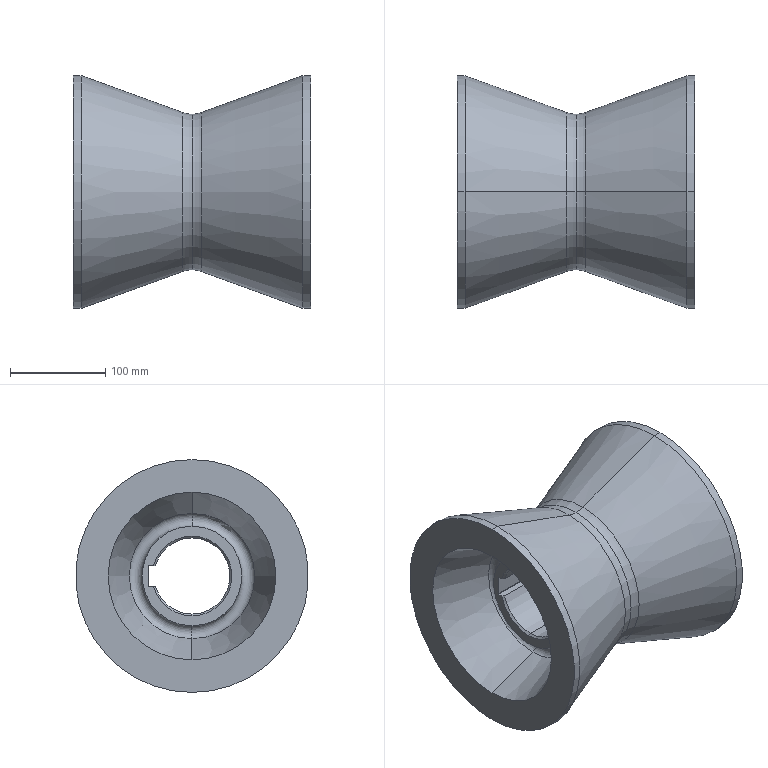Part | SolidWorks | features Chamfer 1, Fillet 1, ICE 1, Revolution 1 | 1 solid | 42 faces | box 250 x 245 x 245 mm | volume 5466955 mm3 | cone 14 | cylinder 13 | torus 8 | plane 7 | commonest cylinder face diameters 105 x4 245 x4 80 x3 1 x2
STEP:
#1=CARTESIAN_POINT('',(-10.261,0.,83.735));
#2=VERTEX_POINT('',#1);
#3=CARTESIAN_POINT('',(0.,0.,81.925));
#4=VERTEX_POINT('',#3);
#5=CARTESIAN_POINT('',(0.,0.,111.925));
#6=DIRECTION('',(0.,-1.,0.));
#7=DIRECTION('',(0.,0.,-1.));
#8=AXIS2_PLACEMENT_3D('',#5,#6,#7);
#9=CIRCLE('',#8,30.);
#10=EDGE_CURVE('',#2,#4,#9,.T.);
#11=ORIENTED_EDGE('',*,*,#10,.T.);
#12=CARTESIAN_POINT('',(0.,0.,-81.925));
#13=VERTEX_POINT('',#12);
#14=CARTESIAN_POINT('',(0.,0.,0.));
#15=DIRECTION('',(-1.,0.,0.));
#16=DIRECTION('',(0.,0.,1.));
#17=AXIS2_PLACEMENT_3D('',#14,#15,#16);
#18=CIRCLE('',#17,81.925);
#19=EDGE_CURVE('',#4,#13,#18,.T.);
#20=ORIENTED_EDGE('',*,*,#19,.T.);
#21=CARTESIAN_POINT('',(-10.261,0.,-83.735));
#22=VERTEX_POINT('',#21);
#23=CARTESIAN_POINT('',(0.,0.,-111.925));
#24=DIRECTION('',(0.,1.,0.));
#25=DIRECTION('',(0.,0.,1.));
#26=AXIS2_PLACEMENT_3D('',#23,#24,#25);
#27=CIRCLE('',#26,30.);
#28=EDGE_CURVE('',#22,#13,#27,.T.);
#29=ORIENTED_EDGE('',*,*,#28,.F.);
#30=CARTESIAN_POINT('',(-10.261,0.,0.));
#31=DIRECTION('',(-1.,0.,0.));
#32=DIRECTION('',(0.,0.,1.));
#33=AXIS2_PLACEMENT_3D('',#30,#31,#32);
#34=CIRCLE('',#33,83.735);
#35=EDGE_CURVE('',#2,#22,#34,.T.);
#36=ORIENTED_EDGE('',*,*,#35,.F.);
#37=EDGE_LOOP('',(#11,#20,#29,#36));
#38=FACE_OUTER_BOUND('',#37,.T.);
#39=CARTESIAN_POINT('',(0.,0.,0.));
#40=DIRECTION('',(-1.,0.,0.));
#41=DIRECTION('',(0.,0.,1.));
#42=AXIS2_PLACEMENT_3D('',#39,#40,#41);
#43=TOROIDAL_SURFACE('',#42,111.925,30.);
#44=ADVANCED_FACE('',(#38),#43,.F.);
#45=ORIENTED_EDGE('',*,*,#28,.T.);
#46=CARTESIAN_POINT('',(0.,0.,0.));
#47=DIRECTION('',(-1.,0.,0.));
#48=DIRECTION('',(0.,0.,1.));
#49=AXIS2_PLACEMENT_3D('',#46,#47,#48);
#50=CIRCLE('',#49,81.925);
#51=EDGE_CURVE('',#13,#4,#50,.T.);
#52=ORIENTED_EDGE('',*,*,#51,.T.);
#53=ORIENTED_EDGE('',*,*,#10,.F.);
#54=CARTESIAN_POINT('',(-10.261,0.,0.));
#55=DIRECTION('',(-1.,0.,0.));
#56=DIRECTION('',(0.,0.,1.));
#57=AXIS2_PLACEMENT_3D('',#54,#55,#56);
#58=CIRCLE('',#57,83.735);
#59=EDGE_CURVE('',#22,#2,#58,.T.);
#60=ORIENTED_EDGE('',*,*,#59,.F.);
#61=EDGE_LOOP('',(#45,#52,#53,#60));
#62=FACE_OUTER_BOUND('',#61,.T.);
#63=CARTESIAN_POINT('',(0.,0.,0.));
#64=DIRECTION('',(-1.,0.,0.));
#65=DIRECTION('',(0.,0.,1.));
#66=AXIS2_PLACEMENT_3D('',#63,#64,#65);
#67=TOROIDAL_SURFACE('',#66,111.925,30.);
#68=ADVANCED_FACE('',(#62),#67,.F.);
#69=CARTESIAN_POINT('',(-68.,0.,-40.));
#70=VERTEX_POINT('',#69);
#71=CARTESIAN_POINT('',(-68.,0.,40.));
#72=VERTEX_POINT('',#71);
#73=CARTESIAN_POINT('',(-68.,0.,0.));
#74=DIRECTION('',(-1.,0.,0.));
#75=DIRECTION('',(0.,0.,-1.));
#76=AXIS2_PLACEMENT_3D('',#73,#74,#75);
#77=CIRCLE('',#76,40.);
#78=EDGE_CURVE('',#70,#72,#77,.T.);
#79=ORIENTED_EDGE('',*,*,#78,.F.);
#80=CARTESIAN_POINT('',(-70.,0.,-42.));
#81=VERTEX_POINT('',#80);
#82=CARTESIAN_POINT('',(-68.,0.,-40.));
#83=DIRECTION('',(-0.7071,0.,-0.7071));
#84=VECTOR('',#83,1000.);
#85=LINE('',#82,#84);
#86=EDGE_CURVE('',#70,#81,#85,.T.);
#87=ORIENTED_EDGE('',*,*,#86,.T.);
#88=CARTESIAN_POINT('',(-70.,0.,42.));
#89=VERTEX_POINT('',#88);
#90=CARTESIAN_POINT('',(-70.,0.,0.));
#91=DIRECTION('',(1.,0.,0.));
#92=DIRECTION('',(0.,0.,-1.));
#93=AXIS2_PLACEMENT_3D('',#90,#91,#92);
#94=CIRCLE('',#93,42.);
#95=EDGE_CURVE('',#89,#81,#94,.T.);
#96=ORIENTED_EDGE('',*,*,#95,.F.);
#97=CARTESIAN_POINT('',(-68.,0.,40.));
#98=DIRECTION('',(-0.7071,0.,0.7071));
#99=VECTOR('',#98,1000.);
#100=LINE('',#97,#99);
#101=EDGE_CURVE('',#72,#89,#100,.T.);
#102=ORIENTED_EDGE('',*,*,#101,.F.);
#103=EDGE_LOOP('',(#79,#87,#96,#102));
#104=FACE_OUTER_BOUND('',#103,.T.);
#105=CARTESIAN_POINT('',(-68.,0.,0.));
#106=DIRECTION('',(-1.,0.,0.));
#107=DIRECTION('',(0.,0.,1.));
#108=AXIS2_PLACEMENT_3D('',#105,#106,#107);
#109=CONICAL_SURFACE('',#108,40.,0.7854);
#110=ADVANCED_FACE('',(#104),#109,.F.);
#111=CARTESIAN_POINT('',(-68.,38.458,11.));
#112=VERTEX_POINT('',#111);
#113=CARTESIAN_POINT('',(-68.,0.,0.));
#114=DIRECTION('',(-1.,0.,0.));
#115=DIRECTION('',(0.,0.,-1.));
#116=AXIS2_PLACEMENT_3D('',#113,#114,#115);
#117=CIRCLE('',#116,40.);
#118=EDGE_CURVE('',#72,#112,#117,.T.);
#119=ORIENTED_EDGE('',*,*,#118,.F.);
#120=ORIENTED_EDGE('',*,*,#101,.T.);
#121=CARTESIAN_POINT('',(-70.,40.534,11.));
#122=VERTEX_POINT('',#121);
#123=CARTESIAN_POINT('',(-70.,0.,0.));
#124=DIRECTION('',(1.,0.,0.));
#125=DIRECTION('',(0.,0.,-1.));
#126=AXIS2_PLACEMENT_3D('',#123,#124,#125);
#127=CIRCLE('',#126,42.);
#128=EDGE_CURVE('',#122,#89,#127,.T.);
#129=ORIENTED_EDGE('',*,*,#128,.F.);
#130=CARTESIAN_POINT('',(-68.,38.458,11.));
#131=CARTESIAN_POINT('',(-68.666,39.15,11.));
#132=CARTESIAN_POINT('',(-69.333,39.842,11.));
#133=CARTESIAN_POINT('',(-70.,40.534,11.));
#134=B_SPLINE_CURVE_WITH_KNOTS('',3,(#130,#131,#132,#133),.UNSPECIFIED.,.F.,.F.,(4,4),(0.,0.002883),.UNSPECIFIED.);
#135=EDGE_CURVE('',#112,#122,#134,.T.);
#136=ORIENTED_EDGE('',*,*,#135,.F.);
#137=EDGE_LOOP('',(#119,#120,#129,#136));
#138=FACE_OUTER_BOUND('',#137,.T.);
#139=CARTESIAN_POINT('',(-68.,0.,0.));
#140=DIRECTION('',(-1.,0.,0.));
#141=DIRECTION('',(0.,0.,1.));
#142=AXIS2_PLACEMENT_3D('',#139,#140,#141);
#143=CONICAL_SURFACE('',#142,40.,0.7854);
#144=ADVANCED_FACE('',(#138),#143,.F.);
#145=CARTESIAN_POINT('',(68.,0.,40.));
#146=VERTEX_POINT('',#145);
#147=CARTESIAN_POINT('',(68.,0.,-40.));
#148=VERTEX_POINT('',#147);
#149=CARTESIAN_POINT('',(68.,0.,0.));
#150=DIRECTION('',(1.,0.,0.));
#151=DIRECTION('',(0.,0.,1.));
#152=AXIS2_PLACEMENT_3D('',#149,#150,#151);
#153=CIRCLE('',#152,40.);
#154=EDGE_CURVE('',#146,#148,#153,.T.);
#155=ORIENTED_EDGE('',*,*,#154,.F.);
#156=CARTESIAN_POINT('',(70.,0.,42.));
#157=VERTEX_POINT('',#156);
#158=CARTESIAN_POINT('',(70.,0.,42.));
#159=DIRECTION('',(0.7071,0.,0.7071));
#160=VECTOR('',#159,1000.);
#161=LINE('',#158,#160);
#162=EDGE_CURVE('',#146,#157,#161,.T.);
#163=ORIENTED_EDGE('',*,*,#162,.T.);
#164=CARTESIAN_POINT('',(70.,0.,-42.));
#165=VERTEX_POINT('',#164);
#166=CARTESIAN_POINT('',(70.,0.,0.));
#167=DIRECTION('',(-1.,0.,0.));
#168=DIRECTION('',(0.,0.,1.));
#169=AXIS2_PLACEMENT_3D('',#166,#167,#168);
#170=CIRCLE('',#169,42.);
#171=EDGE_CURVE('',#165,#157,#170,.T.);
#172=ORIENTED_EDGE('',*,*,#171,.F.);
#173=CARTESIAN_POINT('',(70.,0.,-42.));
#174=DIRECTION('',(0.7071,0.,-0.7071));
#175=VECTOR('',#174,1000.);
#176=LINE('',#173,#175);
#177=EDGE_CURVE('',#148,#165,#176,.T.);
#178=ORIENTED_EDGE('',*,*,#177,.F.);
#179=EDGE_LOOP('',(#155,#163,#172,#178));
#180=FACE_OUTER_BOUND('',#179,.T.);
#181=CARTESIAN_POINT('',(70.,0.,0.));
#182=DIRECTION('',(1.,0.,0.));
#183=DIRECTION('',(0.,0.,-1.));
#184=AXIS2_PLACEMENT_3D('',#181,#182,#183);
#185=CONICAL_SURFACE('',#184,42.,0.7854);
#186=ADVANCED_FACE('',(#180),#185,.F.);
#187=CARTESIAN_POINT('',(68.,38.458,-11.));
#188=VERTEX_POINT('',#187);
#189=CARTESIAN_POINT('',(68.,0.,0.));
#190=DIRECTION('',(1.,0.,0.));
#191=DIRECTION('',(0.,0.,1.));
#192=AXIS2_PLACEMENT_3D('',#189,#190,#191);
#193=CIRCLE('',#192,40.);
#194=EDGE_CURVE('',#148,#188,#193,.T.);
#195=ORIENTED_EDGE('',*,*,#194,.F.);
#196=ORIENTED_EDGE('',*,*,#177,.T.);
#197=CARTESIAN_POINT('',(70.,40.534,-11.));
#198=VERTEX_POINT('',#197);
#199=CARTESIAN_POINT('',(70.,0.,0.));
#200=DIRECTION('',(-1.,0.,0.));
#201=DIRECTION('',(0.,0.,1.));
#202=AXIS2_PLACEMENT_3D('',#199,#200,#201);
#203=CIRCLE('',#202,42.);
#204=EDGE_CURVE('',#198,#165,#203,.T.);
#205=ORIENTED_EDGE('',*,*,#204,.F.);
#206=CARTESIAN_POINT('',(68.,38.458,-11.));
#207=CARTESIAN_POINT('',(68.666,39.15,-11.));
#208=CARTESIAN_POINT('',(69.333,39.842,-11.));
#209=CARTESIAN_POINT('',(70.,40.534,-11.));
#210=B_SPLINE_CURVE_WITH_KNOTS('',3,(#206,#207,#208,#209),.UNSPECIFIED.,.F.,.F.,(4,4),(0.,0.002883),.UNSPECIFIED.);
#211=EDGE_CURVE('',#188,#198,#210,.T.);
#212=ORIENTED_EDGE('',*,*,#211,.F.);
#213=EDGE_LOOP('',(#195,#196,#205,#212));
#214=FACE_OUTER_BOUND('',#213,.T.);
#215=CARTESIAN_POINT('',(70.,0.,0.));
#216=DIRECTION('',(1.,0.,0.));
#217=DIRECTION('',(0.,0.,-1.));
#218=AXIS2_PLACEMENT_3D('',#215,#216,#217);
#219=CONICAL_SURFACE('',#218,42.,0.7854);
#220=ADVANCED_FACE('',(#214),#219,.F.);
#221=ORIENTED_EDGE('',*,*,#154,.T.);
#222=CARTESIAN_POINT('',(125.,0.,-40.));
#223=DIRECTION('',(-1.,0.,0.));
#224=VECTOR('',#223,1000.);
#225=LINE('',#222,#224);
#226=EDGE_CURVE('',#148,#70,#225,.T.);
#227=ORIENTED_EDGE('',*,*,#226,.T.);
#228=ORIENTED_EDGE('',*,*,#78,.T.);
#229=CARTESIAN_POINT('',(125.,0.,40.));
#230=DIRECTION('',(-1.,0.,0.));
#231=VECTOR('',#230,1000.);
#232=LINE('',#229,#231);
#233=EDGE_CURVE('',#146,#72,#232,.T.);
#234=ORIENTED_EDGE('',*,*,#233,.F.);
#235=EDGE_LOOP('',(#221,#227,#228,#234));
#236=FACE_OUTER_BOUND('',#235,.T.);
#237=CARTESIAN_POINT('',(125.,0.,0.));
#238=DIRECTION('',(-1.,0.,0.));
#239=DIRECTION('',(0.,0.,1.));
#240=AXIS2_PLACEMENT_3D('',#237,#238,#239);
#241=CYLINDRICAL_SURFACE('',#240,40.);
#242=ADVANCED_FACE('',(#236),#241,.F.);
#243=CARTESIAN_POINT('',(68.,38.458,11.));
#244=VERTEX_POINT('',#243);
#245=CARTESIAN_POINT('',(68.,0.,0.));
#246=DIRECTION('',(1.,0.,0.));
#247=DIRECTION('',(0.,0.,1.));
#248=AXIS2_PLACEMENT_3D('',#245,#246,#247);
#249=CIRCLE('',#248,40.);
#250=EDGE_CURVE('',#244,#146,#249,.T.);
#251=ORIENTED_EDGE('',*,*,#250,.T.);
#252=ORIENTED_EDGE('',*,*,#233,.T.);
#253=ORIENTED_EDGE('',*,*,#118,.T.);
#254=CARTESIAN_POINT('',(125.,38.458,11.));
#255=DIRECTION('',(-1.,0.,0.));
#256=VECTOR('',#255,1000.);
#257=LINE('',#254,#256);
#258=EDGE_CURVE('',#244,#112,#257,.T.);
#259=ORIENTED_EDGE('',*,*,#258,.F.);
#260=EDGE_LOOP('',(#251,#252,#253,#259));
#261=FACE_OUTER_BOUND('',#260,.T.);
#262=CARTESIAN_POINT('',(125.,0.,0.));
#263=DIRECTION('',(-1.,0.,0.));
#264=DIRECTION('',(0.,0.,1.));
#265=AXIS2_PLACEMENT_3D('',#262,#263,#264);
#266=CYLINDRICAL_SURFACE('',#265,40.);
#267=ADVANCED_FACE('',(#261),#266,.F.);
#268=CARTESIAN_POINT('',(-66.476,0.,-52.5));
#269=VERTEX_POINT('',#268);
#270=CARTESIAN_POINT('',(-66.476,0.,52.5));
#271=VERTEX_POINT('',#270);
#272=CARTESIAN_POINT('',(-66.476,0.,0.));
#273=DIRECTION('',(-1.,0.,0.));
#274=DIRECTION('',(0.,0.,1.));
#275=AXIS2_PLACEMENT_3D('',#272,#273,#274);
#276=CIRCLE('',#275,52.5);
#277=EDGE_CURVE('',#269,#271,#276,.T.);
#278=ORIENTED_EDGE('',*,*,#277,.F.);
#279=CARTESIAN_POINT('',(-64.082,0.,-66.078));
#280=VERTEX_POINT('',#279);
#281=CARTESIAN_POINT('',(-66.476,0.,-59.5));
#282=DIRECTION('',(0.,1.,0.));
#283=DIRECTION('',(0.,0.,1.));
#284=AXIS2_PLACEMENT_3D('',#281,#282,#283);
#285=CIRCLE('',#284,7.);
#286=EDGE_CURVE('',#269,#280,#285,.T.);
#287=ORIENTED_EDGE('',*,*,#286,.T.);
#288=CARTESIAN_POINT('',(-64.082,0.,66.078));
#289=VERTEX_POINT('',#288);
#290=CARTESIAN_POINT('',(-64.082,0.,0.));
#291=DIRECTION('',(-1.,0.,0.));
#292=DIRECTION('',(0.,0.,1.));
#293=AXIS2_PLACEMENT_3D('',#290,#291,#292);
#294=CIRCLE('',#293,66.078);
#295=EDGE_CURVE('',#280,#289,#294,.T.);
#296=ORIENTED_EDGE('',*,*,#295,.T.);
#297=CARTESIAN_POINT('',(-66.476,0.,59.5));
#298=DIRECTION('',(0.,-1.,0.));
#299=DIRECTION('',(0.,0.,-1.));
#300=AXIS2_PLACEMENT_3D('',#297,#298,#299);
#301=CIRCLE('',#300,7.);
#302=EDGE_CURVE('',#271,#289,#301,.T.);
#303=ORIENTED_EDGE('',*,*,#302,.F.);
#304=EDGE_LOOP('',(#278,#287,#296,#303));
#305=FACE_OUTER_BOUND('',#304,.T.);
#306=CARTESIAN_POINT('',(-66.476,0.,0.));
#307=DIRECTION('',(-1.,0.,0.));
#308=DIRECTION('',(0.,0.,1.));
#309=AXIS2_PLACEMENT_3D('',#306,#307,#308);
#310=TOROIDAL_SURFACE('',#309,59.5,7.);
#311=ADVANCED_FACE('',(#305),#310,.F.);
#312=ORIENTED_EDGE('',*,*,#295,.F.);
#313=CARTESIAN_POINT('',(-125.,0.,-88.25));
#314=VERTEX_POINT('',#313);
#315=CARTESIAN_POINT('',(-125.,0.,-88.25));
#316=DIRECTION('',(-0.9397,0.,-0.342));
#317=VECTOR('',#316,1000.);
#318=LINE('',#315,#317);
#319=EDGE_CURVE('',#280,#314,#318,.T.);
#320=ORIENTED_EDGE('',*,*,#319,.T.);
#321=CARTESIAN_POINT('',(-125.,0.,88.25));
#322=VERTEX_POINT('',#321);
#323=CARTESIAN_POINT('',(-125.,0.,0.));
#324=DIRECTION('',(-1.,0.,0.));
#325=DIRECTION('',(0.,0.,1.));
#326=AXIS2_PLACEMENT_3D('',#323,#324,#325);
#327=CIRCLE('',#326,88.25);
#328=EDGE_CURVE('',#314,#322,#327,.T.);
#329=ORIENTED_EDGE('',*,*,#328,.T.);
#330=CARTESIAN_POINT('',(-125.,0.,88.25));
#331=DIRECTION('',(-0.9397,0.,0.342));
#332=VECTOR('',#331,1000.);
#333=LINE('',#330,#332);
#334=EDGE_CURVE('',#289,#322,#333,.T.);
#335=ORIENTED_EDGE('',*,*,#334,.F.);
#336=EDGE_LOOP('',(#312,#320,#329,#335));
#337=FACE_OUTER_BOUND('',#336,.T.);
#338=CARTESIAN_POINT('',(-125.,0.,0.));
#339=DIRECTION('',(-1.,0.,0.));
#340=DIRECTION('',(0.,0.,1.));
#341=AXIS2_PLACEMENT_3D('',#338,#339,#340);
#342=CONICAL_SURFACE('',#341,88.25,0.3491);
#343=ADVANCED_FACE('',(#337),#342,.F.);
#344=CARTESIAN_POINT('',(-116.768,0.,122.5));
#345=VERTEX_POINT('',#344);
#346=CARTESIAN_POINT('',(-116.768,0.,-122.5));
#347=VERTEX_POINT('',#346);
#348=CARTESIAN_POINT('',(-116.768,0.,0.));
#349=DIRECTION('',(-1.,0.,0.));
#350=DIRECTION('',(0.,0.,1.));
#351=AXIS2_PLACEMENT_3D('',#348,#349,#350);
#352=CIRCLE('',#351,122.5);
#353=EDGE_CURVE('',#345,#347,#352,.T.);
#354=ORIENTED_EDGE('',*,*,#353,.T.);
#355=CARTESIAN_POINT('',(-125.,0.,-122.5));
#356=VERTEX_POINT('',#355);
#357=CARTESIAN_POINT('',(-70.,0.,-122.5));
#358=DIRECTION('',(-1.,0.,0.));
#359=VECTOR('',#358,1000.);
#360=LINE('',#357,#359);
#361=EDGE_CURVE('',#347,#356,#360,.T.);
#362=ORIENTED_EDGE('',*,*,#361,.T.);
#363=CARTESIAN_POINT('',(-125.,0.,122.5));
#364=VERTEX_POINT('',#363);
#365=CARTESIAN_POINT('',(-125.,0.,0.));
#366=DIRECTION('',(-1.,0.,0.));
#367=DIRECTION('',(0.,0.,1.));
#368=AXIS2_PLACEMENT_3D('',#365,#366,#367);
#369=CIRCLE('',#368,122.5);
#370=EDGE_CURVE('',#364,#356,#369,.T.);
#371=ORIENTED_EDGE('',*,*,#370,.F.);
#372=CARTESIAN_POINT('',(-70.,0.,122.5));
#373=DIRECTION('',(-1.,0.,0.));
#374=VECTOR('',#373,1000.);
#375=LINE('',#372,#374);
#376=EDGE_CURVE('',#345,#364,#375,.T.);
#377=ORIENTED_EDGE('',*,*,#376,.F.);
#378=EDGE_LOOP('',(#354,#362,#371,#377));
#379=FACE_OUTER_BOUND('',#378,.T.);
#380=CARTESIAN_POINT('',(-70.,0.,0.));
#381=DIRECTION('',(-1.,0.,0.));
#382=DIRECTION('',(0.,0.,1.));
#383=AXIS2_PLACEMENT_3D('',#380,#381,#382);
#384=CYLINDRICAL_SURFACE('',#383,122.5);
#385=ADVANCED_FACE('',(#379),#384,.T.);
#386=ORIENTED_EDGE('',*,*,#35,.T.);
#387=CARTESIAN_POINT('',(-10.261,0.,-83.735));
#388=DIRECTION('',(-0.9397,0.,-0.342));
#389=VECTOR('',#388,1000.);
#390=LINE('',#387,#389);
#391=EDGE_CURVE('',#22,#347,#390,.T.);
#392=ORIENTED_EDGE('',*,*,#391,.T.);
#393=ORIENTED_EDGE('',*,*,#353,.F.);
#394=CARTESIAN_POINT('',(-10.261,0.,83.735));
#395=DIRECTION('',(-0.9397,0.,0.342));
#396=VECTOR('',#395,1000.);
#397=LINE('',#394,#396);
#398=EDGE_CURVE('',#2,#345,#397,.T.);
#399=ORIENTED_EDGE('',*,*,#398,.F.);
#400=EDGE_LOOP('',(#386,#392,#393,#399));
#401=FACE_OUTER_BOUND('',#400,.T.);
#402=CARTESIAN_POINT('',(-10.261,0.,0.));
#403=DIRECTION('',(-1.,0.,0.));
#404=DIRECTION('',(0.,0.,1.));
#405=AXIS2_PLACEMENT_3D('',#402,#403,#404);
#406=CONICAL_SURFACE('',#405,83.735,0.3491);
#407=ADVANCED_FACE('',(#401),#406,.T.);
#408=ORIENTED_EDGE('',*,*,#51,.F.);
#409=CARTESIAN_POINT('',(10.261,0.,-83.735));
#410=VERTEX_POINT('',#409);
#411=CARTESIAN_POINT('',(0.,0.,-111.925));
#412=DIRECTION('',(0.,1.,0.));
#413=DIRECTION('',(0.,0.,1.));
#414=AXIS2_PLACEMENT_3D('',#411,#412,#413);
#415=CIRCLE('',#414,30.);
#416=EDGE_CURVE('',#13,#410,#415,.T.);
#417=ORIENTED_EDGE('',*,*,#416,.T.);
#418=CARTESIAN_POINT('',(10.261,0.,83.735));
#419=VERTEX_POINT('',#418);
#420=CARTESIAN_POINT('',(10.261,0.,0.));
#421=DIRECTION('',(-1.,0.,0.));
#422=DIRECTION('',(0.,0.,1.));
#423=AXIS2_PLACEMENT_3D('',#420,#421,#422);
#424=CIRCLE('',#423,83.735);
#425=EDGE_CURVE('',#410,#419,#424,.T.);
#426=ORIENTED_EDGE('',*,*,#425,.T.);
#427=CARTESIAN_POINT('',(0.,0.,111.925));
#428=DIRECTION('',(0.,-1.,0.));
#429=DIRECTION('',(0.,0.,-1.));
#430=AXIS2_PLACEMENT_3D('',#427,#428,#429);
#431=CIRCLE('',#430,30.);
#432=EDGE_CURVE('',#4,#419,#431,.T.);
#433=ORIENTED_EDGE('',*,*,#432,.F.);
#434=EDGE_LOOP('',(#408,#417,#426,#433));
#435=FACE_OUTER_BOUND('',#434,.T.);
#436=CARTESIAN_POINT('',(0.,0.,0.));
#437=DIRECTION('',(-1.,0.,0.));
#438=DIRECTION('',(0.,0.,1.));
#439=AXIS2_PLACEMENT_3D('',#436,#437,#438);
#440=TOROIDAL_SURFACE('',#439,111.925,30.);
#441=ADVANCED_FACE('',(#435),#440,.F.);
#442=CARTESIAN_POINT('',(10.261,0.,0.));
#443=DIRECTION('',(-1.,0.,0.));
#444=DIRECTION('',(0.,0.,1.));
#445=AXIS2_PLACEMENT_3D('',#442,#443,#444);
#446=CIRCLE('',#445,83.735);
#447=EDGE_CURVE('',#419,#410,#446,.T.);
#448=ORIENTED_EDGE('',*,*,#447,.F.);
#449=CARTESIAN_POINT('',(116.768,0.,122.5));
#450=VERTEX_POINT('',#449);
#451=CARTESIAN_POINT('',(116.768,0.,122.5));
#452=DIRECTION('',(0.9397,0.,0.342));
#453=VECTOR('',#452,1000.);
#454=LINE('',#451,#453);
#455=EDGE_CURVE('',#419,#450,#454,.T.);
#456=ORIENTED_EDGE('',*,*,#455,.T.);
#457=CARTESIAN_POINT('',(116.768,0.,-122.5));
#458=VERTEX_POINT('',#457);
#459=CARTESIAN_POINT('',(116.768,0.,0.));
#460=DIRECTION('',(-1.,0.,0.));
#461=DIRECTION('',(0.,0.,1.));
#462=AXIS2_PLACEMENT_3D('',#459,#460,#461);
#463=CIRCLE('',#462,122.5);
#464=EDGE_CURVE('',#450,#458,#463,.T.);
#465=ORIENTED_EDGE('',*,*,#464,.T.);
#466=CARTESIAN_POINT('',(116.768,0.,-122.5));
#467=DIRECTION('',(0.9397,0.,-0.342));
#468=VECTOR('',#467,1000.);
#469=LINE('',#466,#468);
#470=EDGE_CURVE('',#410,#458,#469,.T.);
#471=ORIENTED_EDGE('',*,*,#470,.F.);
#472=EDGE_LOOP('',(#448,#456,#465,#471));
#473=FACE_OUTER_BOUND('',#472,.T.);
#474=CARTESIAN_POINT('',(116.768,0.,0.));
#475=DIRECTION('',(1.,0.,0.));
#476=DIRECTION('',(0.,0.,-1.));
#477=AXIS2_PLACEMENT_3D('',#474,#475,#476);
#478=CONICAL_SURFACE('',#477,122.5,0.3491);
#479=ADVANCED_FACE('',(#473),#478,.T.);
#480=CARTESIAN_POINT('',(125.,0.,122.5));
#481=VERTEX_POINT('',#480);
#482=CARTESIAN_POINT('',(125.,0.,-122.5));
#483=VERTEX_POINT('',#482);
#484=CARTESIAN_POINT('',(125.,0.,0.));
#485=DIRECTION('',(-1.,0.,0.));
#486=DIRECTION('',(0.,0.,1.));
#487=AXIS2_PLACEMENT_3D('',#484,#485,#486);
#488=CIRCLE('',#487,122.5);
#489=EDGE_CURVE('',#481,#483,#488,.T.);
#490=ORIENTED_EDGE('',*,*,#489,.T.);
#491=CARTESIAN_POINT('',(-70.,0.,-122.5));
#492=DIRECTION('',(-1.,0.,0.));
#493=VECTOR('',#492,1000.);
#494=LINE('',#491,#493);
#495=EDGE_CURVE('',#483,#458,#494,.T.);
#496=ORIENTED_EDGE('',*,*,#495,.T.);
#497=ORIENTED_EDGE('',*,*,#464,.F.);
#498=CARTESIAN_POINT('',(-70.,0.,122.5));
#499=DIRECTION('',(-1.,0.,0.));
#500=VECTOR('',#499,1000.);
#501=LINE('',#498,#500);
#502=EDGE_CURVE('',#481,#450,#501,.T.);
#503=ORIENTED_EDGE('',*,*,#502,.F.);
#504=EDGE_LOOP('',(#490,#496,#497,#503));
#505=FACE_OUTER_BOUND('',#504,.T.);
#506=CARTESIAN_POINT('',(-70.,0.,0.));
#507=DIRECTION('',(-1.,0.,0.));
#508=DIRECTION('',(0.,0.,1.));
#509=AXIS2_PLACEMENT_3D('',#506,#507,#508);
#510=CYLINDRICAL_SURFACE('',#509,122.5);
#511=ADVANCED_FACE('',(#505),#510,.T.);
#512=CARTESIAN_POINT('',(64.082,0.,-66.078));
#513=VERTEX_POINT('',#512);
#514=CARTESIAN_POINT('',(64.082,0.,66.078));
#515=VERTEX_POINT('',#514);
#516=CARTESIAN_POINT('',(64.082,0.,0.));
#517=DIRECTION('',(-1.,0.,0.));
#518=DIRECTION('',(0.,0.,1.));
#519=AXIS2_PLACEMENT_3D('',#516,#517,#518);
#520=CIRCLE('',#519,66.078);
#521=EDGE_CURVE('',#513,#515,#520,.T.);
#522=ORIENTED_EDGE('',*,*,#521,.T.);
#523=CARTESIAN_POINT('',(125.,0.,88.25));
#524=VERTEX_POINT('',#523);
#525=CARTESIAN_POINT('',(64.082,0.,66.078));
#526=DIRECTION('',(0.9397,0.,0.342));
#527=VECTOR('',#526,1000.);
#528=LINE('',#525,#527);
#529=EDGE_CURVE('',#515,#524,#528,.T.);
#530=ORIENTED_EDGE('',*,*,#529,.T.);
#531=CARTESIAN_POINT('',(125.,0.,-88.25));
#532=VERTEX_POINT('',#531);
#533=CARTESIAN_POINT('',(125.,0.,0.));
#534=DIRECTION('',(-1.,0.,0.));
#535=DIRECTION('',(0.,0.,1.));
#536=AXIS2_PLACEMENT_3D('',#533,#534,#535);
#537=CIRCLE('',#536,88.25);
#538=EDGE_CURVE('',#532,#524,#537,.T.);
#539=ORIENTED_EDGE('',*,*,#538,.F.);
#540=CARTESIAN_POINT('',(64.082,0.,-66.078));
#541=DIRECTION('',(0.9397,0.,-0.342));
#542=VECTOR('',#541,1000.);
#543=LINE('',#540,#542);
#544=EDGE_CURVE('',#513,#532,#543,.T.);
#545=ORIENTED_EDGE('',*,*,#544,.F.);
#546=EDGE_LOOP('',(#522,#530,#539,#545));
#547=FACE_OUTER_BOUND('',#546,.T.);
#548=CARTESIAN_POINT('',(64.082,0.,0.));
#549=DIRECTION('',(1.,0.,0.));
#550=DIRECTION('',(0.,0.,-1.));
#551=AXIS2_PLACEMENT_3D('',#548,#549,#550);
#552=CONICAL_SURFACE('',#551,66.078,0.3491);
#553=ADVANCED_FACE('',(#547),#552,.F.);
#554=ORIENTED_EDGE('',*,*,#521,.F.);
#555=CARTESIAN_POINT('',(66.476,0.,-52.5));
#556=VERTEX_POINT('',#555);
#557=CARTESIAN_POINT('',(66.476,0.,-59.5));
#558=DIRECTION('',(0.,1.,0.));
#559=DIRECTION('',(0.,0.,1.));
#560=AXIS2_PLACEMENT_3D('',#557,#558,#559);
#561=CIRCLE('',#560,7.);
#562=EDGE_CURVE('',#513,#556,#561,.T.);
#563=ORIENTED_EDGE('',*,*,#562,.T.);
#564=CARTESIAN_POINT('',(66.476,0.,52.5));
#565=VERTEX_POINT('',#564);
#566=CARTESIAN_POINT('',(66.476,0.,0.));
#567=DIRECTION('',(-1.,0.,0.));
#568=DIRECTION('',(0.,0.,1.));
#569=AXIS2_PLACEMENT_3D('',#566,#567,#568);
#570=CIRCLE('',#569,52.5);
#571=EDGE_CURVE('',#556,#565,#570,.T.);
#572=ORIENTED_EDGE('',*,*,#571,.T.);
#573=CARTESIAN_POINT('',(66.476,0.,59.5));
#574=DIRECTION('',(0.,-1.,0.));
#575=DIRECTION('',(0.,0.,-1.));
#576=AXIS2_PLACEMENT_3D('',#573,#574,#575);
#577=CIRCLE('',#576,7.);
#578=EDGE_CURVE('',#515,#565,#577,.T.);
#579=ORIENTED_EDGE('',*,*,#578,.F.);
#580=EDGE_LOOP('',(#554,#563,#572,#579));
#581=FACE_OUTER_BOUND('',#580,.T.);
#582=CARTESIAN_POINT('',(66.476,0.,0.));
#583=DIRECTION('',(-1.,0.,0.));
#584=DIRECTION('',(0.,0.,1.));
#585=AXIS2_PLACEMENT_3D('',#582,#583,#584);
#586=TOROIDAL_SURFACE('',#585,59.5,7.);
#587=ADVANCED_FACE('',(#581),#586,.F.);
#588=CARTESIAN_POINT('',(70.,0.,52.5));
#589=VERTEX_POINT('',#588);
#590=CARTESIAN_POINT('',(70.,0.,-52.5));
#591=VERTEX_POINT('',#590);
#592=CARTESIAN_POINT('',(70.,0.,0.));
#593=DIRECTION('',(-1.,0.,0.));
#594=DIRECTION('',(0.,0.,1.));
#595=AXIS2_PLACEMENT_3D('',#592,#593,#594);
#596=CIRCLE('',#595,52.5);
#597=EDGE_CURVE('',#589,#591,#596,.T.);
#598=ORIENTED_EDGE('',*,*,#597,.T.);
#599=CARTESIAN_POINT('',(-70.,0.,-52.5));
#600=DIRECTION('',(-1.,0.,0.));
#601=VECTOR('',#600,1000.);
#602=LINE('',#599,#601);
#603=EDGE_CURVE('',#591,#556,#602,.T.);
#604=ORIENTED_EDGE('',*,*,#603,.T.);
#605=CARTESIAN_POINT('',(66.476,0.,0.));
#606=DIRECTION('',(-1.,0.,0.));
#607=DIRECTION('',(0.,0.,1.));
#608=AXIS2_PLACEMENT_3D('',#605,#606,#607);
#609=CIRCLE('',#608,52.5);
#610=EDGE_CURVE('',#565,#556,#609,.T.);
#611=ORIENTED_EDGE('',*,*,#610,.F.);
#612=CARTESIAN_POINT('',(-70.,0.,52.5));
#613=DIRECTION('',(-1.,0.,0.));
#614=VECTOR('',#613,1000.);
#615=LINE('',#612,#614);
#616=EDGE_CURVE('',#589,#565,#615,.T.);
#617=ORIENTED_EDGE('',*,*,#616,.F.);
#618=EDGE_LOOP('',(#598,#604,#611,#617));
#619=FACE_OUTER_BOUND('',#618,.T.);
#620=CARTESIAN_POINT('',(-70.,0.,0.));
#621=DIRECTION('',(-1.,0.,0.));
#622=DIRECTION('',(0.,0.,1.));
#623=AXIS2_PLACEMENT_3D('',#620,#621,#622);
#624=CYLINDRICAL_SURFACE('',#623,52.5);
#625=ADVANCED_FACE('',(#619),#624,.T.);
#626=CARTESIAN_POINT('',(-66.476,0.,0.));
#627=DIRECTION('',(-1.,0.,0.));
#628=DIRECTION('',(0.,0.,1.));
#629=AXIS2_PLACEMENT_3D('',#626,#627,#628);
#630=CIRCLE('',#629,52.5);
#631=EDGE_CURVE('',#271,#269,#630,.T.);
#632=ORIENTED_EDGE('',*,*,#631,.T.);
#633=CARTESIAN_POINT('',(-70.,0.,-52.5));
#634=VERTEX_POINT('',#633);
#635=CARTESIAN_POINT('',(-70.,0.,-52.5));
#636=DIRECTION('',(-1.,0.,0.));
#637=VECTOR('',#636,1000.);
#638=LINE('',#635,#637);
#639=EDGE_CURVE('',#269,#634,#638,.T.);
#640=ORIENTED_EDGE('',*,*,#639,.T.);
#641=CARTESIAN_POINT('',(-70.,0.,52.5));
#642=VERTEX_POINT('',#641);
#643=CARTESIAN_POINT('',(-70.,0.,0.));
#644=DIRECTION('',(-1.,0.,0.));
#645=DIRECTION('',(0.,0.,1.));
#646=AXIS2_PLACEMENT_3D('',#643,#644,#645);
#647=CIRCLE('',#646,52.5);
#648=EDGE_CURVE('',#642,#634,#647,.T.);
#649=ORIENTED_EDGE('',*,*,#648,.F.);
#650=CARTESIAN_POINT('',(-70.,0.,52.5));
#651=DIRECTION('',(-1.,0.,0.));
#652=VECTOR('',#651,1000.);
#653=LINE('',#650,#652);
#654=EDGE_CURVE('',#271,#642,#653,.T.);
#655=ORIENTED_EDGE('',*,*,#654,.F.);
#656=EDGE_LOOP('',(#632,#640,#649,#655));
#657=FACE_OUTER_BOUND('',#656,.T.);
#658=CARTESIAN_POINT('',(-70.,0.,0.));
#659=DIRECTION('',(-1.,0.,0.));
#660=DIRECTION('',(0.,0.,1.));
#661=AXIS2_PLACEMENT_3D('',#658,#659,#660);
#662=CYLINDRICAL_SURFACE('',#661,52.5);
#663=ADVANCED_FACE('',(#657),#662,.T.);
#664=ORIENTED_EDGE('',*,*,#639,.F.);
#665=ORIENTED_EDGE('',*,*,#277,.T.);
#666=ORIENTED_EDGE('',*,*,#654,.T.);
#667=CARTESIAN_POINT('',(-70.,0.,0.));
#668=DIRECTION('',(-1.,0.,0.));
#669=DIRECTION('',(0.,0.,1.));
#670=AXIS2_PLACEMENT_3D('',#667,#668,#669);
#671=CIRCLE('',#670,52.5);
#672=EDGE_CURVE('',#634,#642,#671,.T.);
#673=ORIENTED_EDGE('',*,*,#672,.F.);
#674=EDGE_LOOP('',(#664,#665,#666,#673));
#675=FACE_OUTER_BOUND('',#674,.T.);
#676=CARTESIAN_POINT('',(-70.,0.,0.));
#677=DIRECTION('',(-1.,0.,0.));
#678=DIRECTION('',(0.,0.,1.));
#679=AXIS2_PLACEMENT_3D('',#676,#677,#678);
#680=CYLINDRICAL_SURFACE('',#679,52.5);
#681=ADVANCED_FACE('',(#675),#680,.T.);
#682=CARTESIAN_POINT('',(-70.,44.9,11.));
#683=VERTEX_POINT('',#682);
#684=CARTESIAN_POINT('',(-70.,45.4,11.));
#685=DIRECTION('',(0.,1.,0.));
#686=VECTOR('',#685,1000.);
#687=LINE('',#684,#686);
#688=EDGE_CURVE('',#122,#683,#687,.T.);
#689=ORIENTED_EDGE('',*,*,#688,.F.);
#690=ORIENTED_EDGE('',*,*,#128,.T.);
#691=ORIENTED_EDGE('',*,*,#95,.T.);
#692=CARTESIAN_POINT('',(-70.,40.534,-11.));
#693=VERTEX_POINT('',#692);
#694=CARTESIAN_POINT('',(-70.,0.,0.));
#695=DIRECTION('',(1.,0.,0.));
#696=DIRECTION('',(0.,0.,-1.));
#697=AXIS2_PLACEMENT_3D('',#694,#695,#696);
#698=CIRCLE('',#697,42.);
#699=EDGE_CURVE('',#81,#693,#698,.T.);
#700=ORIENTED_EDGE('',*,*,#699,.T.);
#701=CARTESIAN_POINT('',(-70.,44.9,-11.));
#702=VERTEX_POINT('',#701);
#703=CARTESIAN_POINT('',(-70.,45.4,-11.));
#704=DIRECTION('',(0.,-1.,0.));
#705=VECTOR('',#704,1000.);
#706=LINE('',#703,#705);
#707=EDGE_CURVE('',#702,#693,#706,.T.);
#708=ORIENTED_EDGE('',*,*,#707,.F.);
#709=CARTESIAN_POINT('',(-70.,45.4,-10.5));
#710=VERTEX_POINT('',#709);
#711=CARTESIAN_POINT('',(-70.,44.9,-10.5));
#712=DIRECTION('',(1.,0.,0.));
#713=DIRECTION('',(0.,0.,-1.));
#714=AXIS2_PLACEMENT_3D('',#711,#712,#713);
#715=CIRCLE('',#714,0.5);
#716=EDGE_CURVE('',#702,#710,#715,.T.);
#717=ORIENTED_EDGE('',*,*,#716,.T.);
#718=CARTESIAN_POINT('',(-70.,45.4,10.5));
#719=VERTEX_POINT('',#718);
#720=CARTESIAN_POINT('',(-70.,45.4,-11.));
#721=DIRECTION('',(0.,0.,-1.));
#722=VECTOR('',#721,1000.);
#723=LINE('',#720,#722);
#724=EDGE_CURVE('',#719,#710,#723,.T.);
#725=ORIENTED_EDGE('',*,*,#724,.F.);
#726=CARTESIAN_POINT('',(-70.,44.9,10.5));
#727=DIRECTION('',(1.,0.,0.));
#728=DIRECTION('',(0.,0.,-1.));
#729=AXIS2_PLACEMENT_3D('',#726,#727,#728);
#730=CIRCLE('',#729,0.5);
#731=EDGE_CURVE('',#719,#683,#730,.T.);
#732=ORIENTED_EDGE('',*,*,#731,.T.);
#733=EDGE_LOOP('',(#689,#690,#691,#700,#708,#717,#725,#732));
#734=FACE_BOUND('',#733,.T.);
#735=ORIENTED_EDGE('',*,*,#648,.T.);
#736=ORIENTED_EDGE('',*,*,#672,.T.);
#737=EDGE_LOOP('',(#735,#736));
#738=FACE_OUTER_BOUND('',#737,.T.);
#739=CARTESIAN_POINT('',(-70.,52.5,0.));
#740=DIRECTION('',(1.,0.,0.));
#741=DIRECTION('',(0.,0.,-1.));
#742=AXIS2_PLACEMENT_3D('',#739,#740,#741);
#743=PLANE('',#742);
#744=ADVANCED_FACE('',(#734,#738),#743,.F.);
#745=CARTESIAN_POINT('',(70.,45.4,10.5));
#746=VERTEX_POINT('',#745);
#747=CARTESIAN_POINT('',(70.,45.4,-10.5));
#748=VERTEX_POINT('',#747);
#749=CARTESIAN_POINT('',(70.,45.4,0.));
#750=DIRECTION('',(0.,0.,-1.));
#751=VECTOR('',#750,1000.);
#752=LINE('',#749,#751);
#753=EDGE_CURVE('',#746,#748,#752,.T.);
#754=ORIENTED_EDGE('',*,*,#753,.T.);
#755=CARTESIAN_POINT('',(70.,44.9,-11.));
#756=VERTEX_POINT('',#755);
#757=CARTESIAN_POINT('',(70.,44.9,-10.5));
#758=DIRECTION('',(-1.,0.,0.));
#759=DIRECTION('',(0.,0.,1.));
#760=AXIS2_PLACEMENT_3D('',#757,#758,#759);
#761=CIRCLE('',#760,0.5);
#762=EDGE_CURVE('',#748,#756,#761,.T.);
#763=ORIENTED_EDGE('',*,*,#762,.T.);
#764=CARTESIAN_POINT('',(70.,52.5,-11.));
#765=DIRECTION('',(0.,-1.,0.));
#766=VECTOR('',#765,1000.);
#767=LINE('',#764,#766);
#768=EDGE_CURVE('',#756,#198,#767,.T.);
#769=ORIENTED_EDGE('',*,*,#768,.T.);
#770=ORIENTED_EDGE('',*,*,#204,.T.);
#771=ORIENTED_EDGE('',*,*,#171,.T.);
#772=CARTESIAN_POINT('',(70.,40.534,11.));
#773=VERTEX_POINT('',#772);
#774=CARTESIAN_POINT('',(70.,0.,0.));
#775=DIRECTION('',(-1.,0.,0.));
#776=DIRECTION('',(0.,0.,1.));
#777=AXIS2_PLACEMENT_3D('',#774,#775,#776);
#778=CIRCLE('',#777,42.);
#779=EDGE_CURVE('',#157,#773,#778,.T.);
#780=ORIENTED_EDGE('',*,*,#779,.T.);
#781=CARTESIAN_POINT('',(70.,44.9,11.));
#782=VERTEX_POINT('',#781);
#783=CARTESIAN_POINT('',(70.,52.5,11.));
#784=DIRECTION('',(0.,1.,0.));
#785=VECTOR('',#784,1000.);
#786=LINE('',#783,#785);
#787=EDGE_CURVE('',#773,#782,#786,.T.);
#788=ORIENTED_EDGE('',*,*,#787,.T.);
#789=CARTESIAN_POINT('',(70.,44.9,10.5));
#790=DIRECTION('',(-1.,0.,0.));
#791=DIRECTION('',(0.,0.,1.));
#792=AXIS2_PLACEMENT_3D('',#789,#790,#791);
#793=CIRCLE('',#792,0.5);
#794=EDGE_CURVE('',#782,#746,#793,.T.);
#795=ORIENTED_EDGE('',*,*,#794,.T.);
#796=EDGE_LOOP('',(#754,#763,#769,#770,#771,#780,#788,#795));
#797=FACE_BOUND('',#796,.T.);
#798=ORIENTED_EDGE('',*,*,#597,.F.);
#799=CARTESIAN_POINT('',(70.,0.,0.));
#800=DIRECTION('',(-1.,0.,0.));
#801=DIRECTION('',(0.,0.,1.));
#802=AXIS2_PLACEMENT_3D('',#799,#800,#801);
#803=CIRCLE('',#802,52.5);
#804=EDGE_CURVE('',#591,#589,#803,.T.);
#805=ORIENTED_EDGE('',*,*,#804,.F.);
#806=EDGE_LOOP('',(#798,#805));
#807=FACE_OUTER_BOUND('',#806,.T.);
#808=CARTESIAN_POINT('',(70.,52.5,0.));
#809=DIRECTION('',(-1.,0.,0.));
#810=DIRECTION('',(0.,0.,1.));
#811=AXIS2_PLACEMENT_3D('',#808,#809,#810);
#812=PLANE('',#811);
#813=ADVANCED_FACE('',(#797,#807),#812,.F.);
#814=ORIENTED_EDGE('',*,*,#603,.F.);
#815=ORIENTED_EDGE('',*,*,#804,.T.);
#816=ORIENTED_EDGE('',*,*,#616,.T.);
#817=ORIENTED_EDGE('',*,*,#571,.F.);
#818=EDGE_LOOP('',(#814,#815,#816,#817));
#819=FACE_OUTER_BOUND('',#818,.T.);
#820=CARTESIAN_POINT('',(-70.,0.,0.));
#821=DIRECTION('',(-1.,0.,0.));
#822=DIRECTION('',(0.,0.,1.));
#823=AXIS2_PLACEMENT_3D('',#820,#821,#822);
#824=CYLINDRICAL_SURFACE('',#823,52.5);
#825=ADVANCED_FACE('',(#819),#824,.T.);
#826=ORIENTED_EDGE('',*,*,#562,.F.);
#827=CARTESIAN_POINT('',(64.082,0.,0.));
#828=DIRECTION('',(-1.,0.,0.));
#829=DIRECTION('',(0.,0.,1.));
#830=AXIS2_PLACEMENT_3D('',#827,#828,#829);
#831=CIRCLE('',#830,66.078);
#832=EDGE_CURVE('',#515,#513,#831,.T.);
#833=ORIENTED_EDGE('',*,*,#832,.F.);
#834=ORIENTED_EDGE('',*,*,#578,.T.);
#835=ORIENTED_EDGE('',*,*,#610,.T.);
#836=EDGE_LOOP('',(#826,#833,#834,#835));
#837=FACE_OUTER_BOUND('',#836,.T.);
#838=CARTESIAN_POINT('',(66.476,0.,0.));
#839=DIRECTION('',(-1.,0.,0.));
#840=DIRECTION('',(0.,0.,1.));
#841=AXIS2_PLACEMENT_3D('',#838,#839,#840);
#842=TOROIDAL_SURFACE('',#841,59.5,7.);
#843=ADVANCED_FACE('',(#837),#842,.F.);
#844=ORIENTED_EDGE('',*,*,#529,.F.);
#845=ORIENTED_EDGE('',*,*,#832,.T.);
#846=ORIENTED_EDGE('',*,*,#544,.T.);
#847=CARTESIAN_POINT('',(125.,0.,0.));
#848=DIRECTION('',(-1.,0.,0.));
#849=DIRECTION('',(0.,0.,1.));
#850=AXIS2_PLACEMENT_3D('',#847,#848,#849);
#851=CIRCLE('',#850,88.25);
#852=EDGE_CURVE('',#524,#532,#851,.T.);
#853=ORIENTED_EDGE('',*,*,#852,.F.);
#854=EDGE_LOOP('',(#844,#845,#846,#853));
#855=FACE_OUTER_BOUND('',#854,.T.);
#856=CARTESIAN_POINT('',(64.082,0.,0.));
#857=DIRECTION('',(1.,0.,0.));
#858=DIRECTION('',(0.,0.,-1.));
#859=AXIS2_PLACEMENT_3D('',#856,#857,#858);
#860=CONICAL_SURFACE('',#859,66.078,0.3491);
#861=ADVANCED_FACE('',(#855),#860,.F.);
#862=ORIENTED_EDGE('',*,*,#489,.F.);
#863=CARTESIAN_POINT('',(125.,0.,0.));
#864=DIRECTION('',(-1.,0.,0.));
#865=DIRECTION('',(0.,0.,1.));
#866=AXIS2_PLACEMENT_3D('',#863,#864,#865);
#867=CIRCLE('',#866,122.5);
#868=EDGE_CURVE('',#483,#481,#867,.T.);
#869=ORIENTED_EDGE('',*,*,#868,.F.);
#870=EDGE_LOOP('',(#862,#869));
#871=FACE_OUTER_BOUND('',#870,.T.);
#872=ORIENTED_EDGE('',*,*,#538,.T.);
#873=ORIENTED_EDGE('',*,*,#852,.T.);
#874=EDGE_LOOP('',(#872,#873));
#875=FACE_BOUND('',#874,.T.);
#876=CARTESIAN_POINT('',(125.,122.5,0.));
#877=DIRECTION('',(-1.,0.,0.));
#878=DIRECTION('',(0.,0.,1.));
#879=AXIS2_PLACEMENT_3D('',#876,#877,#878);
#880=PLANE('',#879);
#881=ADVANCED_FACE('',(#871,#875),#880,.F.);
#882=ORIENTED_EDGE('',*,*,#495,.F.);
#883=ORIENTED_EDGE('',*,*,#868,.T.);
#884=ORIENTED_EDGE('',*,*,#502,.T.);
#885=CARTESIAN_POINT('',(116.768,0.,0.));
#886=DIRECTION('',(-1.,0.,0.));
#887=DIRECTION('',(0.,0.,1.));
#888=AXIS2_PLACEMENT_3D('',#885,#886,#887);
#889=CIRCLE('',#888,122.5);
#890=EDGE_CURVE('',#458,#450,#889,.T.);
#891=ORIENTED_EDGE('',*,*,#890,.F.);
#892=EDGE_LOOP('',(#882,#883,#884,#891));
#893=FACE_OUTER_BOUND('',#892,.T.);
#894=CARTESIAN_POINT('',(-70.,0.,0.));
#895=DIRECTION('',(-1.,0.,0.));
#896=DIRECTION('',(0.,0.,1.));
#897=AXIS2_PLACEMENT_3D('',#894,#895,#896);
#898=CYLINDRICAL_SURFACE('',#897,122.5);
#899=ADVANCED_FACE('',(#893),#898,.T.);
#900=ORIENTED_EDGE('',*,*,#455,.F.);
#901=ORIENTED_EDGE('',*,*,#425,.F.);
#902=ORIENTED_EDGE('',*,*,#470,.T.);
#903=ORIENTED_EDGE('',*,*,#890,.T.);
#904=EDGE_LOOP('',(#900,#901,#902,#903));
#905=FACE_OUTER_BOUND('',#904,.T.);
#906=CARTESIAN_POINT('',(116.768,0.,0.));
#907=DIRECTION('',(1.,0.,0.));
#908=DIRECTION('',(0.,0.,-1.));
#909=AXIS2_PLACEMENT_3D('',#906,#907,#908);
#910=CONICAL_SURFACE('',#909,122.5,0.3491);
#911=ADVANCED_FACE('',(#905),#910,.T.);
#912=ORIENTED_EDGE('',*,*,#19,.F.);
#913=ORIENTED_EDGE('',*,*,#432,.T.);
#914=ORIENTED_EDGE('',*,*,#447,.T.);
#915=ORIENTED_EDGE('',*,*,#416,.F.);
#916=EDGE_LOOP('',(#912,#913,#914,#915));
#917=FACE_OUTER_BOUND('',#916,.T.);
#918=CARTESIAN_POINT('',(0.,0.,0.));
#919=DIRECTION('',(-1.,0.,0.));
#920=DIRECTION('',(0.,0.,1.));
#921=AXIS2_PLACEMENT_3D('',#918,#919,#920);
#922=TOROIDAL_SURFACE('',#921,111.925,30.);
#923=ADVANCED_FACE('',(#917),#922,.F.);
#924=ORIENTED_EDGE('',*,*,#391,.F.);
#925=ORIENTED_EDGE('',*,*,#59,.T.);
#926=ORIENTED_EDGE('',*,*,#398,.T.);
#927=CARTESIAN_POINT('',(-116.768,0.,0.));
#928=DIRECTION('',(-1.,0.,0.));
#929=DIRECTION('',(0.,0.,1.));
#930=AXIS2_PLACEMENT_3D('',#927,#928,#929);
#931=CIRCLE('',#930,122.5);
#932=EDGE_CURVE('',#347,#345,#931,.T.);
#933=ORIENTED_EDGE('',*,*,#932,.F.);
#934=EDGE_LOOP('',(#924,#925,#926,#933));
#935=FACE_OUTER_BOUND('',#934,.T.);
#936=CARTESIAN_POINT('',(-10.261,0.,0.));
#937=DIRECTION('',(-1.,0.,0.));
#938=DIRECTION('',(0.,0.,1.));
#939=AXIS2_PLACEMENT_3D('',#936,#937,#938);
#940=CONICAL_SURFACE('',#939,83.735,0.3491);
#941=ADVANCED_FACE('',(#935),#940,.T.);
#942=ORIENTED_EDGE('',*,*,#361,.F.);
#943=ORIENTED_EDGE('',*,*,#932,.T.);
#944=ORIENTED_EDGE('',*,*,#376,.T.);
#945=CARTESIAN_POINT('',(-125.,0.,0.));
#946=DIRECTION('',(-1.,0.,0.));
#947=DIRECTION('',(0.,0.,1.));
#948=AXIS2_PLACEMENT_3D('',#945,#946,#947);
#949=CIRCLE('',#948,122.5);
#950=EDGE_CURVE('',#356,#364,#949,.T.);
#951=ORIENTED_EDGE('',*,*,#950,.F.);
#952=EDGE_LOOP('',(#942,#943,#944,#951));
#953=FACE_OUTER_BOUND('',#952,.T.);
#954=CARTESIAN_POINT('',(-70.,0.,0.));
#955=DIRECTION('',(-1.,0.,0.));
#956=DIRECTION('',(0.,0.,1.));
#957=AXIS2_PLACEMENT_3D('',#954,#955,#956);
#958=CYLINDRICAL_SURFACE('',#957,122.5);
#959=ADVANCED_FACE('',(#953),#958,.T.);
#960=CARTESIAN_POINT('',(-125.,0.,0.));
#961=DIRECTION('',(-1.,0.,0.));
#962=DIRECTION('',(0.,0.,1.));
#963=AXIS2_PLACEMENT_3D('',#960,#961,#962);
#964=CIRCLE('',#963,88.25);
#965=EDGE_CURVE('',#322,#314,#964,.T.);
#966=ORIENTED_EDGE('',*,*,#965,.F.);
#967=ORIENTED_EDGE('',*,*,#328,.F.);
#968=EDGE_LOOP('',(#966,#967));
#969=FACE_BOUND('',#968,.T.);
#970=ORIENTED_EDGE('',*,*,#370,.T.);
#971=ORIENTED_EDGE('',*,*,#950,.T.);
#972=EDGE_LOOP('',(#970,#971));
#973=FACE_OUTER_BOUND('',#972,.T.);
#974=CARTESIAN_POINT('',(-125.,122.5,0.));
#975=DIRECTION('',(1.,0.,0.));
#976=DIRECTION('',(0.,0.,-1.));
#977=AXIS2_PLACEMENT_3D('',#974,#975,#976);
#978=PLANE('',#977);
#979=ADVANCED_FACE('',(#969,#973),#978,.F.);
#980=ORIENTED_EDGE('',*,*,#319,.F.);
#981=CARTESIAN_POINT('',(-64.082,0.,0.));
#982=DIRECTION('',(-1.,0.,0.));
#983=DIRECTION('',(0.,0.,1.));
#984=AXIS2_PLACEMENT_3D('',#981,#982,#983);
#985=CIRCLE('',#984,66.078);
#986=EDGE_CURVE('',#289,#280,#985,.T.);
#987=ORIENTED_EDGE('',*,*,#986,.F.);
#988=ORIENTED_EDGE('',*,*,#334,.T.);
#989=ORIENTED_EDGE('',*,*,#965,.T.);
#990=EDGE_LOOP('',(#980,#987,#988,#989));
#991=FACE_OUTER_BOUND('',#990,.T.);
#992=CARTESIAN_POINT('',(-125.,0.,0.));
#993=DIRECTION('',(-1.,0.,0.));
#994=DIRECTION('',(0.,0.,1.));
#995=AXIS2_PLACEMENT_3D('',#992,#993,#994);
#996=CONICAL_SURFACE('',#995,88.25,0.3491);
#997=ADVANCED_FACE('',(#991),#996,.F.);
#998=ORIENTED_EDGE('',*,*,#286,.F.);
#999=ORIENTED_EDGE('',*,*,#631,.F.);
#1000=ORIENTED_EDGE('',*,*,#302,.T.);
#1001=ORIENTED_EDGE('',*,*,#986,.T.);
#1002=EDGE_LOOP('',(#998,#999,#1000,#1001));
#1003=FACE_OUTER_BOUND('',#1002,.T.);
#1004=CARTESIAN_POINT('',(-66.476,0.,0.));
#1005=DIRECTION('',(-1.,0.,0.));
#1006=DIRECTION('',(0.,0.,1.));
#1007=AXIS2_PLACEMENT_3D('',#1004,#1005,#1006);
#1008=TOROIDAL_SURFACE('',#1007,59.5,7.);
#1009=ADVANCED_FACE('',(#1003),#1008,.F.);
#1010=ORIENTED_EDGE('',*,*,#226,.F.);
#1011=ORIENTED_EDGE('',*,*,#194,.T.);
#1012=CARTESIAN_POINT('',(-68.,38.458,-11.));
#1013=VERTEX_POINT('',#1012);
#1014=CARTESIAN_POINT('',(125.,38.458,-11.));
#1015=DIRECTION('',(-1.,0.,0.));
#1016=VECTOR('',#1015,1000.);
#1017=LINE('',#1014,#1016);
#1018=EDGE_CURVE('',#188,#1013,#1017,.T.);
#1019=ORIENTED_EDGE('',*,*,#1018,.T.);
#1020=CARTESIAN_POINT('',(-68.,0.,0.));
#1021=DIRECTION('',(-1.,0.,0.));
#1022=DIRECTION('',(0.,0.,-1.));
#1023=AXIS2_PLACEMENT_3D('',#1020,#1021,#1022);
#1024=CIRCLE('',#1023,40.);
#1025=EDGE_CURVE('',#1013,#70,#1024,.T.);
#1026=ORIENTED_EDGE('',*,*,#1025,.T.);
#1027=EDGE_LOOP('',(#1010,#1011,#1019,#1026));
#1028=FACE_OUTER_BOUND('',#1027,.T.);
#1029=CARTESIAN_POINT('',(125.,0.,0.));
#1030=DIRECTION('',(-1.,0.,0.));
#1031=DIRECTION('',(0.,0.,1.));
#1032=AXIS2_PLACEMENT_3D('',#1029,#1030,#1031);
#1033=CYLINDRICAL_SURFACE('',#1032,40.);
#1034=ADVANCED_FACE('',(#1028),#1033,.F.);
#1035=ORIENTED_EDGE('',*,*,#768,.F.);
#1036=CARTESIAN_POINT('',(-70.,44.9,-11.));
#1037=DIRECTION('',(-1.,0.,0.));
#1038=VECTOR('',#1037,1000.);
#1039=LINE('',#1036,#1038);
#1040=EDGE_CURVE('',#756,#702,#1039,.T.);
#1041=ORIENTED_EDGE('',*,*,#1040,.T.);
#1042=ORIENTED_EDGE('',*,*,#707,.T.);
#1043=CARTESIAN_POINT('',(-70.,40.534,-11.));
#1044=CARTESIAN_POINT('',(-69.333,39.842,-11.));
#1045=CARTESIAN_POINT('',(-68.666,39.15,-11.));
#1046=CARTESIAN_POINT('',(-68.,38.458,-11.));
#1047=B_SPLINE_CURVE_WITH_KNOTS('',3,(#1043,#1044,#1045,#1046),.UNSPECIFIED.,.F.,.F.,(4,4),(0.,0.002883),.UNSPECIFIED.);
#1048=EDGE_CURVE('',#693,#1013,#1047,.T.);
#1049=ORIENTED_EDGE('',*,*,#1048,.T.);
#1050=ORIENTED_EDGE('',*,*,#1018,.F.);
#1051=ORIENTED_EDGE('',*,*,#211,.T.);
#1052=EDGE_LOOP('',(#1035,#1041,#1042,#1049,#1050,#1051));
#1053=FACE_OUTER_BOUND('',#1052,.T.);
#1054=CARTESIAN_POINT('',(125.,45.4,-11.));
#1055=DIRECTION('',(0.,0.,-1.));
#1056=DIRECTION('',(0.,1.,0.));
#1057=AXIS2_PLACEMENT_3D('',#1054,#1055,#1056);
#1058=PLANE('',#1057);
#1059=ADVANCED_FACE('',(#1053),#1058,.F.);
#1060=ORIENTED_EDGE('',*,*,#753,.F.);
#1061=CARTESIAN_POINT('',(-70.,45.4,10.5));
#1062=DIRECTION('',(-1.,0.,0.));
#1063=VECTOR('',#1062,1000.);
#1064=LINE('',#1061,#1063);
#1065=EDGE_CURVE('',#746,#719,#1064,.T.);
#1066=ORIENTED_EDGE('',*,*,#1065,.T.);
#1067=ORIENTED_EDGE('',*,*,#724,.T.);
#1068=CARTESIAN_POINT('',(70.,45.4,-10.5));
#1069=DIRECTION('',(1.,0.,0.));
#1070=VECTOR('',#1069,1000.);
#1071=LINE('',#1068,#1070);
#1072=EDGE_CURVE('',#710,#748,#1071,.T.);
#1073=ORIENTED_EDGE('',*,*,#1072,.T.);
#1074=EDGE_LOOP('',(#1060,#1066,#1067,#1073));
#1075=FACE_OUTER_BOUND('',#1074,.T.);
#1076=CARTESIAN_POINT('',(125.,45.4,-11.));
#1077=DIRECTION('',(0.,1.,0.));
#1078=DIRECTION('',(0.,0.,1.));
#1079=AXIS2_PLACEMENT_3D('',#1076,#1077,#1078);
#1080=PLANE('',#1079);
#1081=ADVANCED_FACE('',(#1075),#1080,.F.);
#1082=ORIENTED_EDGE('',*,*,#688,.T.);
#1083=CARTESIAN_POINT('',(70.,44.9,11.));
#1084=DIRECTION('',(1.,0.,0.));
#1085=VECTOR('',#1084,1000.);
#1086=LINE('',#1083,#1085);
#1087=EDGE_CURVE('',#683,#782,#1086,.T.);
#1088=ORIENTED_EDGE('',*,*,#1087,.T.);
#1089=ORIENTED_EDGE('',*,*,#787,.F.);
#1090=CARTESIAN_POINT('',(70.,40.534,11.));
#1091=CARTESIAN_POINT('',(69.333,39.842,11.));
#1092=CARTESIAN_POINT('',(68.666,39.15,11.));
#1093=CARTESIAN_POINT('',(68.,38.458,11.));
#1094=B_SPLINE_CURVE_WITH_KNOTS('',3,(#1090,#1091,#1092,#1093),.UNSPECIFIED.,.F.,.F.,(4,4),(0.,0.002883),.UNSPECIFIED.);
#1095=EDGE_CURVE('',#773,#244,#1094,.T.);
#1096=ORIENTED_EDGE('',*,*,#1095,.T.);
#1097=ORIENTED_EDGE('',*,*,#258,.T.);
#1098=ORIENTED_EDGE('',*,*,#135,.T.);
#1099=EDGE_LOOP('',(#1082,#1088,#1089,#1096,#1097,#1098));
#1100=FACE_OUTER_BOUND('',#1099,.T.);
#1101=CARTESIAN_POINT('',(125.,45.4,11.));
#1102=DIRECTION('',(0.,0.,1.));
#1103=DIRECTION('',(0.,-1.,0.));
#1104=AXIS2_PLACEMENT_3D('',#1101,#1102,#1103);
#1105=PLANE('',#1104);
#1106=ADVANCED_FACE('',(#1100),#1105,.F.);
#1107=ORIENTED_EDGE('',*,*,#162,.F.);
#1108=ORIENTED_EDGE('',*,*,#250,.F.);
#1109=ORIENTED_EDGE('',*,*,#1095,.F.);
#1110=ORIENTED_EDGE('',*,*,#779,.F.);
#1111=EDGE_LOOP('',(#1107,#1108,#1109,#1110));
#1112=FACE_OUTER_BOUND('',#1111,.T.);
#1113=CARTESIAN_POINT('',(70.,0.,0.));
#1114=DIRECTION('',(1.,0.,0.));
#1115=DIRECTION('',(0.,0.,-1.));
#1116=AXIS2_PLACEMENT_3D('',#1113,#1114,#1115);
#1117=CONICAL_SURFACE('',#1116,42.,0.7854);
#1118=ADVANCED_FACE('',(#1112),#1117,.F.);
#1119=ORIENTED_EDGE('',*,*,#86,.F.);
#1120=ORIENTED_EDGE('',*,*,#1025,.F.);
#1121=ORIENTED_EDGE('',*,*,#1048,.F.);
#1122=ORIENTED_EDGE('',*,*,#699,.F.);
#1123=EDGE_LOOP('',(#1119,#1120,#1121,#1122));
#1124=FACE_OUTER_BOUND('',#1123,.T.);
#1125=CARTESIAN_POINT('',(-68.,0.,0.));
#1126=DIRECTION('',(-1.,0.,0.));
#1127=DIRECTION('',(0.,0.,1.));
#1128=AXIS2_PLACEMENT_3D('',#1125,#1126,#1127);
#1129=CONICAL_SURFACE('',#1128,40.,0.7854);
#1130=ADVANCED_FACE('',(#1124),#1129,.F.);
#1131=ORIENTED_EDGE('',*,*,#794,.F.);
#1132=ORIENTED_EDGE('',*,*,#1087,.F.);
#1133=ORIENTED_EDGE('',*,*,#731,.F.);
#1134=ORIENTED_EDGE('',*,*,#1065,.F.);
#1135=EDGE_LOOP('',(#1131,#1132,#1133,#1134));
#1136=FACE_OUTER_BOUND('',#1135,.T.);
#1137=CARTESIAN_POINT('',(125.,44.9,10.5));
#1138=DIRECTION('',(1.,0.,0.));
#1139=DIRECTION('',(0.,0.,-1.));
#1140=AXIS2_PLACEMENT_3D('',#1137,#1138,#1139);
#1141=CYLINDRICAL_SURFACE('',#1140,0.5);
#1142=ADVANCED_FACE('',(#1136),#1141,.F.);
#1143=ORIENTED_EDGE('',*,*,#762,.F.);
#1144=ORIENTED_EDGE('',*,*,#1072,.F.);
#1145=ORIENTED_EDGE('',*,*,#716,.F.);
#1146=ORIENTED_EDGE('',*,*,#1040,.F.);
#1147=EDGE_LOOP('',(#1143,#1144,#1145,#1146));
#1148=FACE_OUTER_BOUND('',#1147,.T.);
#1149=CARTESIAN_POINT('',(125.,44.9,-10.5));
#1150=DIRECTION('',(1.,0.,0.));
#1151=DIRECTION('',(0.,0.,-1.));
#1152=AXIS2_PLACEMENT_3D('',#1149,#1150,#1151);
#1153=CYLINDRICAL_SURFACE('',#1152,0.5);
#1154=ADVANCED_FACE('',(#1148),#1153,.F.);
#1155=CLOSED_SHELL('',(#44,#68,#110,#144,#186,#220,#242,#267,#311,#343,#385,#407,#441,#479,#511,#553,#587,#625,#663,#681,#744,#813,#825,#843,#861,#881,#899,#911,#923,#941,#959,#979,#997,#1009,#1034,#1059,#1081,#1106,#1118,#1130,#1142,#1154));
#1156=MANIFOLD_SOLID_BREP('',#1155);
#1157=CARTESIAN_POINT('',(0.,0.,0.));
#1158=DIRECTION('',(0.,0.,1.));
#1159=DIRECTION('',(1.,0.,0.));
#1160=AXIS2_PLACEMENT_3D('',#1157,#1158,#1159);
#1161=(LENGTH_UNIT()NAMED_UNIT(*)SI_UNIT(.MILLI.,.METRE.));
#1162=UNCERTAINTY_MEASURE_WITH_UNIT(LENGTH_MEASURE(0.00001),#1161,'','');
#1163=(NAMED_UNIT(*)PLANE_ANGLE_UNIT()SI_UNIT($,.RADIAN.));
#1164=(NAMED_UNIT(*)SI_UNIT($,.STERADIAN.)SOLID_ANGLE_UNIT());
#1165=(GEOMETRIC_REPRESENTATION_CONTEXT(3)GLOBAL_UNCERTAINTY_ASSIGNED_CONTEXT((#1162))GLOBAL_UNIT_ASSIGNED_CONTEXT((#1161,#1163,#1164))REPRESENTATION_CONTEXT('',''));
#1166=ADVANCED_BREP_SHAPE_REPRESENTATION('',(#1156,#1160),#1165);